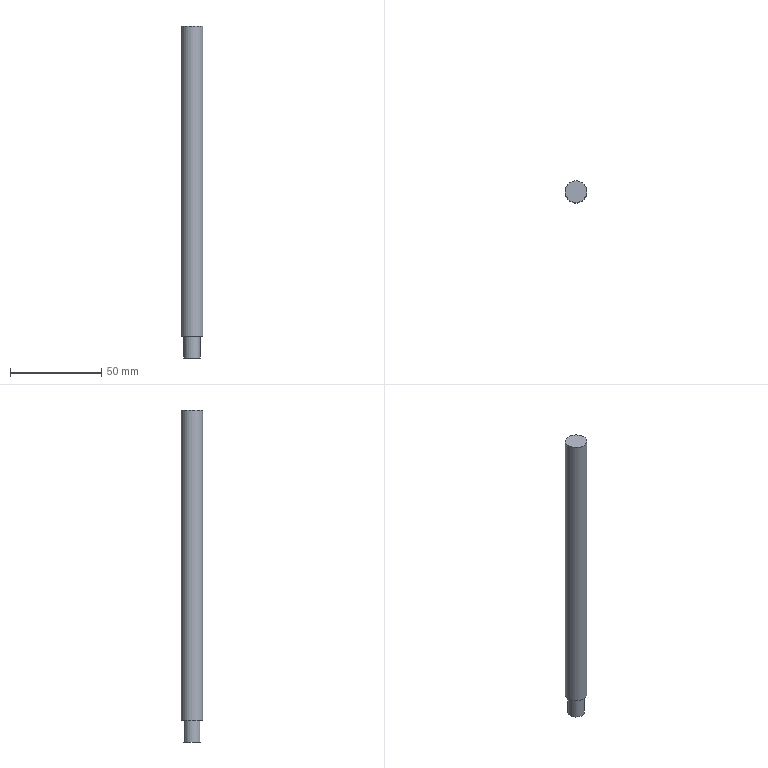Part | STEP file | YBQDJ-YL-8 | 1 solid | 8 faces | box 12 x 12 x 182 mm | volume 19664 mm3 | cylinder 3 | plane 3 | cone 2 | commonest cylinder face diameters 5 x1 9 x1 12 x1
STEP:
#1=CARTESIAN_POINT('',(0.,0.,0.));
#2=DIRECTION('',(0.,0.,1.));
#3=DIRECTION('',(1.,0.,0.));
#4=AXIS2_PLACEMENT_3D('',#1,#2,#3);
#5=CARTESIAN_POINT('',(262.5,-285.,190.));
#6=VERTEX_POINT('',#5);
#7=CARTESIAN_POINT('',(256.5,-285.,190.));
#8=DIRECTION('',(0.,0.,1.));
#9=DIRECTION('',(1.,0.,0.));
#10=AXIS2_PLACEMENT_3D('',#7,#8,#9);
#11=CIRCLE('',#10,6.);
#12=CARTESIAN_POINT('',(256.5,-285.,220.));
#13=DIRECTION('',(0.,0.,-1.));
#14=DIRECTION('',(-1.,0.,0.));
#15=AXIS2_PLACEMENT_3D('',#12,#13,#14);
#16=CYLINDRICAL_SURFACE('',#15,6.);
#17=CARTESIAN_POINT('',(9.425,30.));
#18=DIRECTION('',(-1.,0.));
#19=VECTOR('',#18,1.);
#20=LINE('',#17,#19);
#21=(GEOMETRIC_REPRESENTATION_CONTEXT(2)PARAMETRIC_REPRESENTATION_CONTEXT()REPRESENTATION_CONTEXT('',''));
#22=DEFINITIONAL_REPRESENTATION('',(#20),#21);
#23=PCURVE('',#16,#22);
#24=CARTESIAN_POINT('',(256.5,-285.,190.));
#25=DIRECTION('',(0.,0.,1.));
#26=DIRECTION('',(1.,0.,0.));
#27=AXIS2_PLACEMENT_3D('',#24,#25,#26);
#28=PLANE('',#27);
#29=CARTESIAN_POINT('',(0.,0.));
#30=DIRECTION('',(1.,0.));
#31=AXIS2_PLACEMENT_2D('',#29,#30);
#32=CIRCLE('',#31,6.);
#33=(GEOMETRIC_REPRESENTATION_CONTEXT(2)PARAMETRIC_REPRESENTATION_CONTEXT()REPRESENTATION_CONTEXT('',''));
#34=DEFINITIONAL_REPRESENTATION('',(#32),#33);
#35=PCURVE('',#28,#34);
#36=SURFACE_CURVE('',#11,(#23,#35),.PCURVE_S1.);
#37=EDGE_CURVE('',#6,#6,#36,.T.);
#38=ORIENTED_EDGE('',*,*,#37,.F.);
#39=CARTESIAN_POINT('',(262.5,-285.,20.));
#40=VERTEX_POINT('',#39);
#41=CARTESIAN_POINT('',(262.5,-285.,190.));
#42=CARTESIAN_POINT('',(262.5,-285.,20.));
#43=B_SPLINE_CURVE_WITH_KNOTS('',1,(#41,#42),.UNSPECIFIED.,.F.,.F.,(2,2),(30.,200.),.PIECEWISE_BEZIER_KNOTS.);
#44=CARTESIAN_POINT('',(9.425,0.));
#45=DIRECTION('',(0.,1.));
#46=VECTOR('',#45,1.);
#47=LINE('',#44,#46);
#48=(GEOMETRIC_REPRESENTATION_CONTEXT(2)PARAMETRIC_REPRESENTATION_CONTEXT()REPRESENTATION_CONTEXT('',''));
#49=DEFINITIONAL_REPRESENTATION('',(#47),#48);
#50=PCURVE('',#16,#49);
#51=CARTESIAN_POINT('',(3.142,0.));
#52=DIRECTION('',(0.,1.));
#53=VECTOR('',#52,1.);
#54=LINE('',#51,#53);
#55=(GEOMETRIC_REPRESENTATION_CONTEXT(2)PARAMETRIC_REPRESENTATION_CONTEXT()REPRESENTATION_CONTEXT('',''));
#56=DEFINITIONAL_REPRESENTATION('',(#54),#55);
#57=PCURVE('',#16,#56);
#58=SEAM_CURVE('',#43,(#50,#57),.PCURVE_S1.);
#59=EDGE_CURVE('',#6,#40,#58,.T.);
#60=ORIENTED_EDGE('',*,*,#59,.T.);
#61=CARTESIAN_POINT('',(256.5,-285.,20.));
#62=DIRECTION('',(0.,0.,1.));
#63=DIRECTION('',(1.,0.,0.));
#64=AXIS2_PLACEMENT_3D('',#61,#62,#63);
#65=CIRCLE('',#64,6.);
#66=CARTESIAN_POINT('',(9.425,200.));
#67=DIRECTION('',(-1.,0.));
#68=VECTOR('',#67,1.);
#69=LINE('',#66,#68);
#70=(GEOMETRIC_REPRESENTATION_CONTEXT(2)PARAMETRIC_REPRESENTATION_CONTEXT()REPRESENTATION_CONTEXT('',''));
#71=DEFINITIONAL_REPRESENTATION('',(#69),#70);
#72=PCURVE('',#16,#71);
#73=CARTESIAN_POINT('',(130.5,-90.,20.));
#74=DIRECTION('',(0.,0.,1.));
#75=DIRECTION('',(0.,-1.,0.));
#76=AXIS2_PLACEMENT_3D('',#73,#74,#75);
#77=PLANE('',#76);
#78=CARTESIAN_POINT('',(195.,126.));
#79=DIRECTION('',(0.,1.));
#80=AXIS2_PLACEMENT_2D('',#78,#79);
#81=CIRCLE('',#80,6.);
#82=(GEOMETRIC_REPRESENTATION_CONTEXT(2)PARAMETRIC_REPRESENTATION_CONTEXT()REPRESENTATION_CONTEXT('',''));
#83=DEFINITIONAL_REPRESENTATION('',(#81),#82);
#84=PCURVE('',#77,#83);
#85=SURFACE_CURVE('',#65,(#72,#84),.PCURVE_S1.);
#86=EDGE_CURVE('',#40,#40,#85,.T.);
#87=ORIENTED_EDGE('',*,*,#86,.T.);
#88=ORIENTED_EDGE('',*,*,#59,.F.);
#89=EDGE_LOOP('',(#38,#60,#87,#88));
#90=FACE_BOUND('',#89,.T.);
#91=ADVANCED_FACE('',(#90),#16,.T.);
#92=ORIENTED_EDGE('',*,*,#37,.T.);
#93=EDGE_LOOP('',(#92));
#94=FACE_BOUND('',#93,.T.);
#95=ADVANCED_FACE('',(#94),#28,.T.);
#96=CARTESIAN_POINT('',(252.,-285.,20.));
#97=VERTEX_POINT('',#96);
#98=CARTESIAN_POINT('',(256.5,-285.,20.));
#99=DIRECTION('',(0.,0.,-1.));
#100=DIRECTION('',(-1.,0.,0.));
#101=AXIS2_PLACEMENT_3D('',#98,#99,#100);
#102=CIRCLE('',#101,4.5);
#103=CARTESIAN_POINT('',(195.,121.5));
#104=CARTESIAN_POINT('',(187.206,121.5));
#105=CARTESIAN_POINT('',(191.103,128.25));
#106=CARTESIAN_POINT('',(195.,135.));
#107=CARTESIAN_POINT('',(198.897,128.25));
#108=CARTESIAN_POINT('',(202.794,121.5));
#109=CARTESIAN_POINT('',(195.,121.5));
#110=(BOUNDED_CURVE()B_SPLINE_CURVE(2,(#103,#104,#105,#106,#107,#108,#109),.UNSPECIFIED.,.T.,.F.)B_SPLINE_CURVE_WITH_KNOTS((1,2,2,2,2,1),(-2.094,0.,2.094,4.189,6.283,8.378),.UNSPECIFIED.)CURVE()GEOMETRIC_REPRESENTATION_ITEM()RATIONAL_B_SPLINE_CURVE((1.,0.5,1.,0.5,1.,0.5,1.))REPRESENTATION_ITEM(''));
#111=(GEOMETRIC_REPRESENTATION_CONTEXT(2)PARAMETRIC_REPRESENTATION_CONTEXT()REPRESENTATION_CONTEXT('',''));
#112=DEFINITIONAL_REPRESENTATION('',(#110),#111);
#113=PCURVE('',#77,#112);
#114=CARTESIAN_POINT('',(256.5,-285.,20.));
#115=DIRECTION('',(0.,0.,-1.));
#116=DIRECTION('',(-1.,0.,0.));
#117=AXIS2_PLACEMENT_3D('',#114,#115,#116);
#118=CYLINDRICAL_SURFACE('',#117,4.5);
#119=CARTESIAN_POINT('',(0.,0.));
#120=DIRECTION('',(1.,0.));
#121=VECTOR('',#120,1.);
#122=LINE('',#119,#121);
#123=(GEOMETRIC_REPRESENTATION_CONTEXT(2)PARAMETRIC_REPRESENTATION_CONTEXT()REPRESENTATION_CONTEXT('',''));
#124=DEFINITIONAL_REPRESENTATION('',(#122),#123);
#125=PCURVE('',#118,#124);
#126=SURFACE_CURVE('',#102,(#113,#125),.PCURVE_S1.);
#127=EDGE_CURVE('',#97,#97,#126,.T.);
#128=ORIENTED_EDGE('',*,*,#127,.F.);
#129=EDGE_LOOP('',(#128));
#130=FACE_BOUND('',#129,.T.);
#131=ORIENTED_EDGE('',*,*,#86,.F.);
#132=EDGE_LOOP('',(#131));
#133=FACE_BOUND('',#132,.T.);
#134=ADVANCED_FACE('',(#130,#133),#77,.F.);
#135=ORIENTED_EDGE('',*,*,#127,.T.);
#136=CARTESIAN_POINT('',(252.,-285.,8.));
#137=VERTEX_POINT('',#136);
#138=CARTESIAN_POINT('',(252.,-285.,20.));
#139=CARTESIAN_POINT('',(252.,-285.,8.));
#140=B_SPLINE_CURVE_WITH_KNOTS('',1,(#138,#139),.UNSPECIFIED.,.F.,.F.,(2,2),(0.,12.),.PIECEWISE_BEZIER_KNOTS.);
#141=CARTESIAN_POINT('',(6.283,0.));
#142=DIRECTION('',(0.,1.));
#143=VECTOR('',#142,1.);
#144=LINE('',#141,#143);
#145=(GEOMETRIC_REPRESENTATION_CONTEXT(2)PARAMETRIC_REPRESENTATION_CONTEXT()REPRESENTATION_CONTEXT('',''));
#146=DEFINITIONAL_REPRESENTATION('',(#144),#145);
#147=PCURVE('',#118,#146);
#148=CARTESIAN_POINT('',(0.,0.));
#149=DIRECTION('',(0.,1.));
#150=VECTOR('',#149,1.);
#151=LINE('',#148,#150);
#152=(GEOMETRIC_REPRESENTATION_CONTEXT(2)PARAMETRIC_REPRESENTATION_CONTEXT()REPRESENTATION_CONTEXT('',''));
#153=DEFINITIONAL_REPRESENTATION('',(#151),#152);
#154=PCURVE('',#118,#153);
#155=SEAM_CURVE('',#140,(#147,#154),.PCURVE_S1.);
#156=EDGE_CURVE('',#97,#137,#155,.T.);
#157=ORIENTED_EDGE('',*,*,#156,.T.);
#158=CARTESIAN_POINT('',(256.5,-285.,8.));
#159=DIRECTION('',(0.,0.,-1.));
#160=DIRECTION('',(-1.,0.,0.));
#161=AXIS2_PLACEMENT_3D('',#158,#159,#160);
#162=CIRCLE('',#161,4.5);
#163=CARTESIAN_POINT('',(0.,12.));
#164=DIRECTION('',(1.,0.));
#165=VECTOR('',#164,1.);
#166=LINE('',#163,#165);
#167=(GEOMETRIC_REPRESENTATION_CONTEXT(2)PARAMETRIC_REPRESENTATION_CONTEXT()REPRESENTATION_CONTEXT('',''));
#168=DEFINITIONAL_REPRESENTATION('',(#166),#167);
#169=PCURVE('',#118,#168);
#170=CARTESIAN_POINT('',(256.5,-285.,8.));
#171=DIRECTION('',(0.,0.,-1.));
#172=DIRECTION('',(-1.,0.,0.));
#173=AXIS2_PLACEMENT_3D('',#170,#171,#172);
#174=PLANE('',#173);
#175=CARTESIAN_POINT('',(0.,0.));
#176=DIRECTION('',(1.,0.));
#177=AXIS2_PLACEMENT_2D('',#175,#176);
#178=CIRCLE('',#177,4.5);
#179=(GEOMETRIC_REPRESENTATION_CONTEXT(2)PARAMETRIC_REPRESENTATION_CONTEXT()REPRESENTATION_CONTEXT('',''));
#180=DEFINITIONAL_REPRESENTATION('',(#178),#179);
#181=PCURVE('',#174,#180);
#182=SURFACE_CURVE('',#162,(#169,#181),.PCURVE_S1.);
#183=EDGE_CURVE('',#137,#137,#182,.T.);
#184=ORIENTED_EDGE('',*,*,#183,.F.);
#185=ORIENTED_EDGE('',*,*,#156,.F.);
#186=EDGE_LOOP('',(#135,#157,#184,#185));
#187=FACE_BOUND('',#186,.T.);
#188=ADVANCED_FACE('',(#187),#118,.T.);
#189=CARTESIAN_POINT('',(253.5,-285.,8.));
#190=VERTEX_POINT('',#189);
#191=CARTESIAN_POINT('',(256.5,-285.,8.));
#192=DIRECTION('',(0.,0.,1.));
#193=DIRECTION('',(-1.,0.,0.));
#194=AXIS2_PLACEMENT_3D('',#191,#192,#193);
#195=CIRCLE('',#194,3.);
#196=CARTESIAN_POINT('',(3.,0.));
#197=CARTESIAN_POINT('',(3.,-5.196));
#198=CARTESIAN_POINT('',(-1.5,-2.598));
#199=CARTESIAN_POINT('',(-6.,0.));
#200=CARTESIAN_POINT('',(-1.5,2.598));
#201=CARTESIAN_POINT('',(3.,5.196));
#202=CARTESIAN_POINT('',(3.,0.));
#203=(BOUNDED_CURVE()B_SPLINE_CURVE(2,(#196,#197,#198,#199,#200,#201,#202),.UNSPECIFIED.,.T.,.F.)B_SPLINE_CURVE_WITH_KNOTS((1,2,2,2,2,1),(-2.094,0.,2.094,4.189,6.283,8.378),.UNSPECIFIED.)CURVE()GEOMETRIC_REPRESENTATION_ITEM()RATIONAL_B_SPLINE_CURVE((1.,0.5,1.,0.5,1.,0.5,1.))REPRESENTATION_ITEM(''));
#204=(GEOMETRIC_REPRESENTATION_CONTEXT(2)PARAMETRIC_REPRESENTATION_CONTEXT()REPRESENTATION_CONTEXT('',''));
#205=DEFINITIONAL_REPRESENTATION('',(#203),#204);
#206=PCURVE('',#174,#205);
#207=CARTESIAN_POINT('',(256.5,-285.,8.));
#208=DIRECTION('',(0.,0.,-1.));
#209=DIRECTION('',(-1.,0.,0.));
#210=AXIS2_PLACEMENT_3D('',#207,#208,#209);
#211=CONICAL_SURFACE('',#210,3.,0.7854);
#212=CARTESIAN_POINT('',(6.283,0.));
#213=DIRECTION('',(-1.,0.));
#214=VECTOR('',#213,1.);
#215=LINE('',#212,#214);
#216=(GEOMETRIC_REPRESENTATION_CONTEXT(2)PARAMETRIC_REPRESENTATION_CONTEXT()REPRESENTATION_CONTEXT('',''));
#217=DEFINITIONAL_REPRESENTATION('',(#215),#216);
#218=PCURVE('',#211,#217);
#219=SURFACE_CURVE('',#195,(#206,#218),.PCURVE_S1.);
#220=EDGE_CURVE('',#190,#190,#219,.T.);
#221=ORIENTED_EDGE('',*,*,#220,.T.);
#222=EDGE_LOOP('',(#221));
#223=FACE_BOUND('',#222,.T.);
#224=ORIENTED_EDGE('',*,*,#183,.T.);
#225=EDGE_LOOP('',(#224));
#226=FACE_BOUND('',#225,.T.);
#227=ADVANCED_FACE('',(#223,#226),#174,.T.);
#228=CARTESIAN_POINT('',(254.,-285.,24.));
#229=VERTEX_POINT('',#228);
#230=CARTESIAN_POINT('',(259.,-285.,24.));
#231=VERTEX_POINT('',#230);
#232=CARTESIAN_POINT('',(256.5,-285.,24.));
#233=DIRECTION('',(0.,0.,-1.));
#234=DIRECTION('',(1.,0.,0.));
#235=AXIS2_PLACEMENT_3D('',#232,#233,#234);
#236=CIRCLE('',#235,2.5);
#237=CARTESIAN_POINT('',(256.5,-285.,24.));
#238=DIRECTION('',(0.,0.,-1.));
#239=DIRECTION('',(-1.,0.,0.));
#240=AXIS2_PLACEMENT_3D('',#237,#238,#239);
#241=CONICAL_SURFACE('',#240,2.5,1.03);
#242=CARTESIAN_POINT('',(-3.142,0.));
#243=DIRECTION('',(1.,0.));
#244=VECTOR('',#243,1.);
#245=LINE('',#242,#244);
#246=(GEOMETRIC_REPRESENTATION_CONTEXT(2)PARAMETRIC_REPRESENTATION_CONTEXT()REPRESENTATION_CONTEXT('',''));
#247=DEFINITIONAL_REPRESENTATION('',(#245),#246);
#248=PCURVE('',#241,#247);
#249=CARTESIAN_POINT('',(256.5,-285.,8.));
#250=DIRECTION('',(0.,0.,1.));
#251=DIRECTION('',(1.,0.,0.));
#252=AXIS2_PLACEMENT_3D('',#249,#250,#251);
#253=CYLINDRICAL_SURFACE('',#252,2.5);
#254=CARTESIAN_POINT('',(12.566,16.));
#255=DIRECTION('',(-1.,0.));
#256=VECTOR('',#255,1.);
#257=LINE('',#254,#256);
#258=(GEOMETRIC_REPRESENTATION_CONTEXT(2)PARAMETRIC_REPRESENTATION_CONTEXT()REPRESENTATION_CONTEXT('',''));
#259=DEFINITIONAL_REPRESENTATION('',(#257),#258);
#260=PCURVE('',#253,#259);
#261=SURFACE_CURVE('',#236,(#248,#260),.PCURVE_S1.);
#262=EDGE_CURVE('',#229,#231,#261,.T.);
#263=ORIENTED_EDGE('',*,*,#262,.F.);
#264=CARTESIAN_POINT('',(256.5,-285.,25.502));
#265=VERTEX_POINT('',#264);
#266=CARTESIAN_POINT('',(256.5,-285.,25.502));
#267=CARTESIAN_POINT('',(254.,-285.,24.));
#268=B_SPLINE_CURVE_WITH_KNOTS('',1,(#266,#267),.UNSPECIFIED.,.F.,.F.,(2,2),(-2.917,0.),.PIECEWISE_BEZIER_KNOTS.);
#269=CARTESIAN_POINT('',(0.,0.));
#270=DIRECTION('',(0.,1.));
#271=VECTOR('',#270,1.);
#272=LINE('',#269,#271);
#273=(GEOMETRIC_REPRESENTATION_CONTEXT(2)PARAMETRIC_REPRESENTATION_CONTEXT()REPRESENTATION_CONTEXT('',''));
#274=DEFINITIONAL_REPRESENTATION('',(#272),#273);
#275=PCURVE('',#241,#274);
#276=CARTESIAN_POINT('',(6.283,0.));
#277=DIRECTION('',(0.,1.));
#278=VECTOR('',#277,1.);
#279=LINE('',#276,#278);
#280=(GEOMETRIC_REPRESENTATION_CONTEXT(2)PARAMETRIC_REPRESENTATION_CONTEXT()REPRESENTATION_CONTEXT('',''));
#281=DEFINITIONAL_REPRESENTATION('',(#279),#280);
#282=PCURVE('',#241,#281);
#283=SEAM_CURVE('',#268,(#275,#282),.PCURVE_S1.);
#284=EDGE_CURVE('',#265,#229,#283,.T.);
#285=ORIENTED_EDGE('',*,*,#284,.F.);
#286=ORIENTED_EDGE('',*,*,#284,.T.);
#287=CARTESIAN_POINT('',(256.5,-285.,24.));
#288=DIRECTION('',(0.,0.,-1.));
#289=DIRECTION('',(1.,0.,0.));
#290=AXIS2_PLACEMENT_3D('',#287,#288,#289);
#291=CIRCLE('',#290,2.5);
#292=CARTESIAN_POINT('',(3.142,0.));
#293=DIRECTION('',(1.,0.));
#294=VECTOR('',#293,1.);
#295=LINE('',#292,#294);
#296=(GEOMETRIC_REPRESENTATION_CONTEXT(2)PARAMETRIC_REPRESENTATION_CONTEXT()REPRESENTATION_CONTEXT('',''));
#297=DEFINITIONAL_REPRESENTATION('',(#295),#296);
#298=PCURVE('',#241,#297);
#299=CARTESIAN_POINT('',(6.283,16.));
#300=DIRECTION('',(-1.,0.));
#301=VECTOR('',#300,1.);
#302=LINE('',#299,#301);
#303=(GEOMETRIC_REPRESENTATION_CONTEXT(2)PARAMETRIC_REPRESENTATION_CONTEXT()REPRESENTATION_CONTEXT('',''));
#304=DEFINITIONAL_REPRESENTATION('',(#302),#303);
#305=PCURVE('',#253,#304);
#306=SURFACE_CURVE('',#291,(#298,#305),.PCURVE_S1.);
#307=EDGE_CURVE('',#231,#229,#306,.T.);
#308=ORIENTED_EDGE('',*,*,#307,.F.);
#309=EDGE_LOOP('',(#263,#285,#286,#308));
#310=FACE_BOUND('',#309,.F.);
#311=ADVANCED_FACE('',(#310),#241,.F.);
#312=CARTESIAN_POINT('',(254.,-285.,8.5));
#313=VERTEX_POINT('',#312);
#314=CARTESIAN_POINT('',(256.5,-285.,8.5));
#315=DIRECTION('',(0.,0.,-1.));
#316=DIRECTION('',(-1.,0.,0.));
#317=AXIS2_PLACEMENT_3D('',#314,#315,#316);
#318=CIRCLE('',#317,2.5);
#319=CARTESIAN_POINT('',(9.425,0.5));
#320=DIRECTION('',(-1.,0.));
#321=VECTOR('',#320,1.);
#322=LINE('',#319,#321);
#323=(GEOMETRIC_REPRESENTATION_CONTEXT(2)PARAMETRIC_REPRESENTATION_CONTEXT()REPRESENTATION_CONTEXT('',''));
#324=DEFINITIONAL_REPRESENTATION('',(#322),#323);
#325=PCURVE('',#253,#324);
#326=CARTESIAN_POINT('',(0.,-0.5));
#327=DIRECTION('',(1.,0.));
#328=VECTOR('',#327,1.);
#329=LINE('',#326,#328);
#330=(GEOMETRIC_REPRESENTATION_CONTEXT(2)PARAMETRIC_REPRESENTATION_CONTEXT()REPRESENTATION_CONTEXT('',''));
#331=DEFINITIONAL_REPRESENTATION('',(#329),#330);
#332=PCURVE('',#211,#331);
#333=SURFACE_CURVE('',#318,(#325,#332),.PCURVE_S1.);
#334=EDGE_CURVE('',#313,#313,#333,.T.);
#335=ORIENTED_EDGE('',*,*,#334,.F.);
#336=CARTESIAN_POINT('',(254.,-285.,8.5));
#337=CARTESIAN_POINT('',(254.,-285.,24.));
#338=B_SPLINE_CURVE_WITH_KNOTS('',1,(#336,#337),.UNSPECIFIED.,.F.,.F.,(2,2),(0.5,16.),.PIECEWISE_BEZIER_KNOTS.);
#339=CARTESIAN_POINT('',(9.425,0.));
#340=DIRECTION('',(0.,1.));
#341=VECTOR('',#340,1.);
#342=LINE('',#339,#341);
#343=(GEOMETRIC_REPRESENTATION_CONTEXT(2)PARAMETRIC_REPRESENTATION_CONTEXT()REPRESENTATION_CONTEXT('',''));
#344=DEFINITIONAL_REPRESENTATION('',(#342),#343);
#345=PCURVE('',#253,#344);
#346=CARTESIAN_POINT('',(3.142,0.));
#347=DIRECTION('',(0.,1.));
#348=VECTOR('',#347,1.);
#349=LINE('',#346,#348);
#350=(GEOMETRIC_REPRESENTATION_CONTEXT(2)PARAMETRIC_REPRESENTATION_CONTEXT()REPRESENTATION_CONTEXT('',''));
#351=DEFINITIONAL_REPRESENTATION('',(#349),#350);
#352=PCURVE('',#253,#351);
#353=SEAM_CURVE('',#338,(#345,#352),.PCURVE_S1.);
#354=EDGE_CURVE('',#313,#229,#353,.T.);
#355=ORIENTED_EDGE('',*,*,#354,.T.);
#356=ORIENTED_EDGE('',*,*,#262,.T.);
#357=ORIENTED_EDGE('',*,*,#307,.T.);
#358=ORIENTED_EDGE('',*,*,#354,.F.);
#359=EDGE_LOOP('',(#335,#355,#356,#357,#358));
#360=FACE_BOUND('',#359,.F.);
#361=ADVANCED_FACE('',(#360),#253,.F.);
#362=ORIENTED_EDGE('',*,*,#334,.T.);
#363=CARTESIAN_POINT('',(254.,-285.,8.5));
#364=CARTESIAN_POINT('',(253.5,-285.,8.));
#365=B_SPLINE_CURVE_WITH_KNOTS('',1,(#363,#364),.UNSPECIFIED.,.F.,.F.,(2,2),(-0.7071,0.),.PIECEWISE_BEZIER_KNOTS.);
#366=CARTESIAN_POINT('',(6.283,0.));
#367=DIRECTION('',(0.,1.));
#368=VECTOR('',#367,1.);
#369=LINE('',#366,#368);
#370=(GEOMETRIC_REPRESENTATION_CONTEXT(2)PARAMETRIC_REPRESENTATION_CONTEXT()REPRESENTATION_CONTEXT('',''));
#371=DEFINITIONAL_REPRESENTATION('',(#369),#370);
#372=PCURVE('',#211,#371);
#373=CARTESIAN_POINT('',(0.,0.));
#374=DIRECTION('',(0.,1.));
#375=VECTOR('',#374,1.);
#376=LINE('',#373,#375);
#377=(GEOMETRIC_REPRESENTATION_CONTEXT(2)PARAMETRIC_REPRESENTATION_CONTEXT()REPRESENTATION_CONTEXT('',''));
#378=DEFINITIONAL_REPRESENTATION('',(#376),#377);
#379=PCURVE('',#211,#378);
#380=SEAM_CURVE('',#365,(#372,#379),.PCURVE_S1.);
#381=EDGE_CURVE('',#313,#190,#380,.T.);
#382=ORIENTED_EDGE('',*,*,#381,.T.);
#383=ORIENTED_EDGE('',*,*,#220,.T.);
#384=ORIENTED_EDGE('',*,*,#381,.F.);
#385=EDGE_LOOP('',(#362,#382,#383,#384));
#386=FACE_BOUND('',#385,.F.);
#387=ADVANCED_FACE('',(#386),#211,.F.);
#388=CLOSED_SHELL('',(#91,#95,#134,#188,#227,#311,#361,#387));
#389=MANIFOLD_SOLID_BREP('',#388);
#390=(LENGTH_UNIT()NAMED_UNIT(*)SI_UNIT(.MILLI.,.METRE.));
#391=UNCERTAINTY_MEASURE_WITH_UNIT(LENGTH_MEASURE(0.00001),#390,'','');
#392=(NAMED_UNIT(*)PLANE_ANGLE_UNIT()SI_UNIT($,.RADIAN.));
#393=(NAMED_UNIT(*)SI_UNIT($,.STERADIAN.)SOLID_ANGLE_UNIT());
#394=(GEOMETRIC_REPRESENTATION_CONTEXT(3)GLOBAL_UNCERTAINTY_ASSIGNED_CONTEXT((#391))GLOBAL_UNIT_ASSIGNED_CONTEXT((#390,#392,#393))REPRESENTATION_CONTEXT('',''));
#395=ADVANCED_BREP_SHAPE_REPRESENTATION('',(#4,#389),#394);